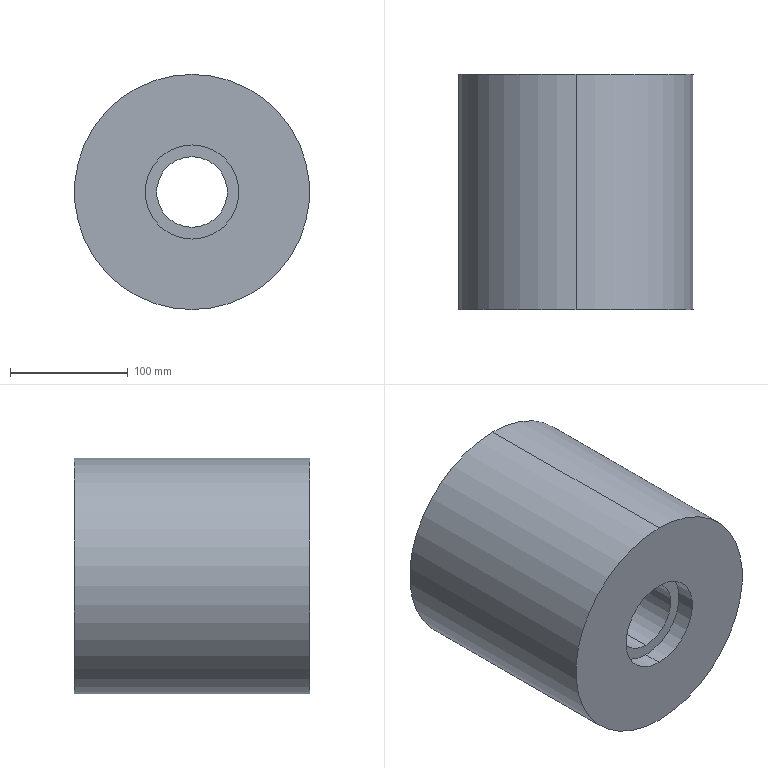Part | SolidWorks | features BaseBody 1 | 1 solid | 12 faces | box 200 x 200 x 200 mm | volume 5647327 mm3 | cylinder 8 | plane 4 | commonest cylinder face diameters 80 x4 60 x2 200 x2
STEP:
#1=CARTESIAN_POINT('',(0.,16.,40.));
#2=VERTEX_POINT('',#1);
#3=CARTESIAN_POINT('',(0.,16.,-40.));
#4=VERTEX_POINT('',#3);
#5=CARTESIAN_POINT('',(0.,16.,0.));
#6=DIRECTION('',(0.,-1.,0.));
#7=DIRECTION('',(0.,0.,-1.));
#8=AXIS2_PLACEMENT_3D('',#5,#6,#7);
#9=CIRCLE('',#8,40.);
#10=EDGE_CURVE('',#2,#4,#9,.T.);
#11=ORIENTED_EDGE('',*,*,#10,.F.);
#12=CARTESIAN_POINT('',(0.,0.,40.));
#13=VERTEX_POINT('',#12);
#14=CARTESIAN_POINT('',(0.,16.,40.));
#15=DIRECTION('',(0.,-1.,0.));
#16=VECTOR('',#15,1000.);
#17=LINE('',#14,#16);
#18=EDGE_CURVE('',#2,#13,#17,.T.);
#19=ORIENTED_EDGE('',*,*,#18,.T.);
#20=CARTESIAN_POINT('',(0.,0.,-40.));
#21=VERTEX_POINT('',#20);
#22=CARTESIAN_POINT('',(0.,0.,0.));
#23=DIRECTION('',(0.,-1.,0.));
#24=DIRECTION('',(0.,0.,-1.));
#25=AXIS2_PLACEMENT_3D('',#22,#23,#24);
#26=CIRCLE('',#25,40.);
#27=EDGE_CURVE('',#13,#21,#26,.T.);
#28=ORIENTED_EDGE('',*,*,#27,.T.);
#29=CARTESIAN_POINT('',(0.,16.,-40.));
#30=DIRECTION('',(0.,-1.,0.));
#31=VECTOR('',#30,1000.);
#32=LINE('',#29,#31);
#33=EDGE_CURVE('',#4,#21,#32,.T.);
#34=ORIENTED_EDGE('',*,*,#33,.F.);
#35=EDGE_LOOP('',(#11,#19,#28,#34));
#36=FACE_OUTER_BOUND('',#35,.T.);
#37=CARTESIAN_POINT('',(0.,16.,0.));
#38=DIRECTION('',(0.,-1.,0.));
#39=DIRECTION('',(0.,0.,-1.));
#40=AXIS2_PLACEMENT_3D('',#37,#38,#39);
#41=CYLINDRICAL_SURFACE('',#40,40.);
#42=ADVANCED_FACE('',(#36),#41,.F.);
#43=CARTESIAN_POINT('',(0.,184.,-40.));
#44=VERTEX_POINT('',#43);
#45=CARTESIAN_POINT('',(0.,184.,40.));
#46=VERTEX_POINT('',#45);
#47=CARTESIAN_POINT('',(0.,184.,0.));
#48=DIRECTION('',(0.,1.,0.));
#49=DIRECTION('',(0.,0.,1.));
#50=AXIS2_PLACEMENT_3D('',#47,#48,#49);
#51=CIRCLE('',#50,40.);
#52=EDGE_CURVE('',#44,#46,#51,.T.);
#53=ORIENTED_EDGE('',*,*,#52,.F.);
#54=CARTESIAN_POINT('',(0.,200.,-40.));
#55=VERTEX_POINT('',#54);
#56=CARTESIAN_POINT('',(0.,184.,-40.));
#57=DIRECTION('',(0.,1.,0.));
#58=VECTOR('',#57,1000.);
#59=LINE('',#56,#58);
#60=EDGE_CURVE('',#44,#55,#59,.T.);
#61=ORIENTED_EDGE('',*,*,#60,.T.);
#62=CARTESIAN_POINT('',(0.,200.,40.));
#63=VERTEX_POINT('',#62);
#64=CARTESIAN_POINT('',(0.,200.,0.));
#65=DIRECTION('',(0.,1.,0.));
#66=DIRECTION('',(0.,0.,1.));
#67=AXIS2_PLACEMENT_3D('',#64,#65,#66);
#68=CIRCLE('',#67,40.);
#69=EDGE_CURVE('',#55,#63,#68,.T.);
#70=ORIENTED_EDGE('',*,*,#69,.T.);
#71=CARTESIAN_POINT('',(0.,184.,40.));
#72=DIRECTION('',(0.,1.,0.));
#73=VECTOR('',#72,1000.);
#74=LINE('',#71,#73);
#75=EDGE_CURVE('',#46,#63,#74,.T.);
#76=ORIENTED_EDGE('',*,*,#75,.F.);
#77=EDGE_LOOP('',(#53,#61,#70,#76));
#78=FACE_OUTER_BOUND('',#77,.T.);
#79=CARTESIAN_POINT('',(0.,184.,0.));
#80=DIRECTION('',(0.,1.,0.));
#81=DIRECTION('',(0.,0.,1.));
#82=AXIS2_PLACEMENT_3D('',#79,#80,#81);
#83=CYLINDRICAL_SURFACE('',#82,40.);
#84=ADVANCED_FACE('',(#78),#83,.F.);
#85=CARTESIAN_POINT('',(0.,200.,100.));
#86=VERTEX_POINT('',#85);
#87=CARTESIAN_POINT('',(0.,200.,-100.));
#88=VERTEX_POINT('',#87);
#89=CARTESIAN_POINT('',(0.,200.,0.));
#90=DIRECTION('',(0.,1.,0.));
#91=DIRECTION('',(0.,0.,1.));
#92=AXIS2_PLACEMENT_3D('',#89,#90,#91);
#93=CIRCLE('',#92,100.);
#94=EDGE_CURVE('',#86,#88,#93,.T.);
#95=ORIENTED_EDGE('',*,*,#94,.F.);
#96=CARTESIAN_POINT('',(0.,0.,100.));
#97=VERTEX_POINT('',#96);
#98=CARTESIAN_POINT('',(0.,200.,100.));
#99=DIRECTION('',(0.,-1.,0.));
#100=VECTOR('',#99,1000.);
#101=LINE('',#98,#100);
#102=EDGE_CURVE('',#86,#97,#101,.T.);
#103=ORIENTED_EDGE('',*,*,#102,.T.);
#104=CARTESIAN_POINT('',(0.,0.,-100.));
#105=VERTEX_POINT('',#104);
#106=CARTESIAN_POINT('',(0.,0.,0.));
#107=DIRECTION('',(0.,1.,0.));
#108=DIRECTION('',(0.,0.,1.));
#109=AXIS2_PLACEMENT_3D('',#106,#107,#108);
#110=CIRCLE('',#109,100.);
#111=EDGE_CURVE('',#97,#105,#110,.T.);
#112=ORIENTED_EDGE('',*,*,#111,.T.);
#113=CARTESIAN_POINT('',(0.,200.,-100.));
#114=DIRECTION('',(0.,-1.,0.));
#115=VECTOR('',#114,1000.);
#116=LINE('',#113,#115);
#117=EDGE_CURVE('',#88,#105,#116,.T.);
#118=ORIENTED_EDGE('',*,*,#117,.F.);
#119=EDGE_LOOP('',(#95,#103,#112,#118));
#120=FACE_OUTER_BOUND('',#119,.T.);
#121=CARTESIAN_POINT('',(0.,200.,0.));
#122=DIRECTION('',(0.,-1.,0.));
#123=DIRECTION('',(0.,0.,-1.));
#124=AXIS2_PLACEMENT_3D('',#121,#122,#123);
#125=CYLINDRICAL_SURFACE('',#124,100.);
#126=ADVANCED_FACE('',(#120),#125,.T.);
#127=CARTESIAN_POINT('',(0.,16.,-30.));
#128=VERTEX_POINT('',#127);
#129=CARTESIAN_POINT('',(0.,16.,30.));
#130=VERTEX_POINT('',#129);
#131=CARTESIAN_POINT('',(0.,16.,0.));
#132=DIRECTION('',(0.,1.,0.));
#133=DIRECTION('',(0.,0.,-1.));
#134=AXIS2_PLACEMENT_3D('',#131,#132,#133);
#135=CIRCLE('',#134,30.);
#136=EDGE_CURVE('',#128,#130,#135,.T.);
#137=ORIENTED_EDGE('',*,*,#136,.F.);
#138=CARTESIAN_POINT('',(0.,184.,-30.));
#139=VERTEX_POINT('',#138);
#140=CARTESIAN_POINT('',(0.,0.,-30.));
#141=DIRECTION('',(0.,1.,0.));
#142=VECTOR('',#141,1000.);
#143=LINE('',#140,#142);
#144=EDGE_CURVE('',#128,#139,#143,.T.);
#145=ORIENTED_EDGE('',*,*,#144,.T.);
#146=CARTESIAN_POINT('',(0.,184.,30.));
#147=VERTEX_POINT('',#146);
#148=CARTESIAN_POINT('',(0.,184.,0.));
#149=DIRECTION('',(0.,-1.,0.));
#150=DIRECTION('',(0.,0.,1.));
#151=AXIS2_PLACEMENT_3D('',#148,#149,#150);
#152=CIRCLE('',#151,30.);
#153=EDGE_CURVE('',#147,#139,#152,.T.);
#154=ORIENTED_EDGE('',*,*,#153,.F.);
#155=CARTESIAN_POINT('',(0.,0.,30.));
#156=DIRECTION('',(0.,1.,0.));
#157=VECTOR('',#156,1000.);
#158=LINE('',#155,#157);
#159=EDGE_CURVE('',#130,#147,#158,.T.);
#160=ORIENTED_EDGE('',*,*,#159,.F.);
#161=EDGE_LOOP('',(#137,#145,#154,#160));
#162=FACE_OUTER_BOUND('',#161,.T.);
#163=CARTESIAN_POINT('',(0.,0.,0.));
#164=DIRECTION('',(0.,1.,0.));
#165=DIRECTION('',(0.,0.,1.));
#166=AXIS2_PLACEMENT_3D('',#163,#164,#165);
#167=CYLINDRICAL_SURFACE('',#166,30.);
#168=ADVANCED_FACE('',(#162),#167,.F.);
#169=ORIENTED_EDGE('',*,*,#144,.F.);
#170=CARTESIAN_POINT('',(0.,16.,0.));
#171=DIRECTION('',(0.,1.,0.));
#172=DIRECTION('',(0.,0.,-1.));
#173=AXIS2_PLACEMENT_3D('',#170,#171,#172);
#174=CIRCLE('',#173,30.);
#175=EDGE_CURVE('',#130,#128,#174,.T.);
#176=ORIENTED_EDGE('',*,*,#175,.F.);
#177=ORIENTED_EDGE('',*,*,#159,.T.);
#178=CARTESIAN_POINT('',(0.,184.,0.));
#179=DIRECTION('',(0.,-1.,0.));
#180=DIRECTION('',(0.,0.,1.));
#181=AXIS2_PLACEMENT_3D('',#178,#179,#180);
#182=CIRCLE('',#181,30.);
#183=EDGE_CURVE('',#139,#147,#182,.T.);
#184=ORIENTED_EDGE('',*,*,#183,.F.);
#185=EDGE_LOOP('',(#169,#176,#177,#184));
#186=FACE_OUTER_BOUND('',#185,.T.);
#187=CARTESIAN_POINT('',(0.,0.,0.));
#188=DIRECTION('',(0.,1.,0.));
#189=DIRECTION('',(0.,0.,1.));
#190=AXIS2_PLACEMENT_3D('',#187,#188,#189);
#191=CYLINDRICAL_SURFACE('',#190,30.);
#192=ADVANCED_FACE('',(#186),#191,.F.);
#193=ORIENTED_EDGE('',*,*,#102,.F.);
#194=CARTESIAN_POINT('',(0.,200.,0.));
#195=DIRECTION('',(0.,1.,0.));
#196=DIRECTION('',(0.,0.,1.));
#197=AXIS2_PLACEMENT_3D('',#194,#195,#196);
#198=CIRCLE('',#197,100.);
#199=EDGE_CURVE('',#88,#86,#198,.T.);
#200=ORIENTED_EDGE('',*,*,#199,.F.);
#201=ORIENTED_EDGE('',*,*,#117,.T.);
#202=CARTESIAN_POINT('',(0.,0.,0.));
#203=DIRECTION('',(0.,1.,0.));
#204=DIRECTION('',(0.,0.,1.));
#205=AXIS2_PLACEMENT_3D('',#202,#203,#204);
#206=CIRCLE('',#205,100.);
#207=EDGE_CURVE('',#105,#97,#206,.T.);
#208=ORIENTED_EDGE('',*,*,#207,.T.);
#209=EDGE_LOOP('',(#193,#200,#201,#208));
#210=FACE_OUTER_BOUND('',#209,.T.);
#211=CARTESIAN_POINT('',(0.,200.,0.));
#212=DIRECTION('',(0.,-1.,0.));
#213=DIRECTION('',(0.,0.,-1.));
#214=AXIS2_PLACEMENT_3D('',#211,#212,#213);
#215=CYLINDRICAL_SURFACE('',#214,100.);
#216=ADVANCED_FACE('',(#210),#215,.T.);
#217=CARTESIAN_POINT('',(0.,200.,0.));
#218=DIRECTION('',(0.,1.,0.));
#219=DIRECTION('',(0.,0.,1.));
#220=AXIS2_PLACEMENT_3D('',#217,#218,#219);
#221=CIRCLE('',#220,40.);
#222=EDGE_CURVE('',#63,#55,#221,.T.);
#223=ORIENTED_EDGE('',*,*,#222,.F.);
#224=ORIENTED_EDGE('',*,*,#69,.F.);
#225=EDGE_LOOP('',(#223,#224));
#226=FACE_BOUND('',#225,.T.);
#227=ORIENTED_EDGE('',*,*,#199,.T.);
#228=ORIENTED_EDGE('',*,*,#94,.T.);
#229=EDGE_LOOP('',(#227,#228));
#230=FACE_OUTER_BOUND('',#229,.T.);
#231=CARTESIAN_POINT('',(0.,200.,0.));
#232=DIRECTION('',(0.,1.,0.));
#233=DIRECTION('',(0.,0.,1.));
#234=AXIS2_PLACEMENT_3D('',#231,#232,#233);
#235=PLANE('',#234);
#236=ADVANCED_FACE('',(#226,#230),#235,.T.);
#237=CARTESIAN_POINT('',(0.,0.,0.));
#238=DIRECTION('',(0.,-1.,0.));
#239=DIRECTION('',(0.,0.,-1.));
#240=AXIS2_PLACEMENT_3D('',#237,#238,#239);
#241=CIRCLE('',#240,40.);
#242=EDGE_CURVE('',#21,#13,#241,.T.);
#243=ORIENTED_EDGE('',*,*,#242,.F.);
#244=ORIENTED_EDGE('',*,*,#27,.F.);
#245=EDGE_LOOP('',(#243,#244));
#246=FACE_BOUND('',#245,.T.);
#247=ORIENTED_EDGE('',*,*,#207,.F.);
#248=ORIENTED_EDGE('',*,*,#111,.F.);
#249=EDGE_LOOP('',(#247,#248));
#250=FACE_OUTER_BOUND('',#249,.T.);
#251=CARTESIAN_POINT('',(0.,0.,0.));
#252=DIRECTION('',(0.,1.,0.));
#253=DIRECTION('',(0.,0.,1.));
#254=AXIS2_PLACEMENT_3D('',#251,#252,#253);
#255=PLANE('',#254);
#256=ADVANCED_FACE('',(#246,#250),#255,.F.);
#257=CARTESIAN_POINT('',(0.,184.,0.));
#258=DIRECTION('',(0.,1.,0.));
#259=DIRECTION('',(0.,0.,1.));
#260=AXIS2_PLACEMENT_3D('',#257,#258,#259);
#261=CIRCLE('',#260,40.);
#262=EDGE_CURVE('',#46,#44,#261,.T.);
#263=ORIENTED_EDGE('',*,*,#262,.T.);
#264=ORIENTED_EDGE('',*,*,#52,.T.);
#265=EDGE_LOOP('',(#263,#264));
#266=FACE_OUTER_BOUND('',#265,.T.);
#267=ORIENTED_EDGE('',*,*,#153,.T.);
#268=ORIENTED_EDGE('',*,*,#183,.T.);
#269=EDGE_LOOP('',(#267,#268));
#270=FACE_BOUND('',#269,.T.);
#271=CARTESIAN_POINT('',(0.,184.,0.));
#272=DIRECTION('',(0.,1.,0.));
#273=DIRECTION('',(0.,0.,1.));
#274=AXIS2_PLACEMENT_3D('',#271,#272,#273);
#275=PLANE('',#274);
#276=ADVANCED_FACE('',(#266,#270),#275,.T.);
#277=ORIENTED_EDGE('',*,*,#60,.F.);
#278=ORIENTED_EDGE('',*,*,#262,.F.);
#279=ORIENTED_EDGE('',*,*,#75,.T.);
#280=ORIENTED_EDGE('',*,*,#222,.T.);
#281=EDGE_LOOP('',(#277,#278,#279,#280));
#282=FACE_OUTER_BOUND('',#281,.T.);
#283=CARTESIAN_POINT('',(0.,184.,0.));
#284=DIRECTION('',(0.,1.,0.));
#285=DIRECTION('',(0.,0.,1.));
#286=AXIS2_PLACEMENT_3D('',#283,#284,#285);
#287=CYLINDRICAL_SURFACE('',#286,40.);
#288=ADVANCED_FACE('',(#282),#287,.F.);
#289=CARTESIAN_POINT('',(0.,16.,0.));
#290=DIRECTION('',(0.,-1.,0.));
#291=DIRECTION('',(0.,0.,-1.));
#292=AXIS2_PLACEMENT_3D('',#289,#290,#291);
#293=CIRCLE('',#292,40.);
#294=EDGE_CURVE('',#4,#2,#293,.T.);
#295=ORIENTED_EDGE('',*,*,#294,.T.);
#296=ORIENTED_EDGE('',*,*,#10,.T.);
#297=EDGE_LOOP('',(#295,#296));
#298=FACE_OUTER_BOUND('',#297,.T.);
#299=ORIENTED_EDGE('',*,*,#175,.T.);
#300=ORIENTED_EDGE('',*,*,#136,.T.);
#301=EDGE_LOOP('',(#299,#300));
#302=FACE_BOUND('',#301,.T.);
#303=CARTESIAN_POINT('',(0.,16.,0.));
#304=DIRECTION('',(0.,-1.,0.));
#305=DIRECTION('',(0.,0.,-1.));
#306=AXIS2_PLACEMENT_3D('',#303,#304,#305);
#307=PLANE('',#306);
#308=ADVANCED_FACE('',(#298,#302),#307,.T.);
#309=ORIENTED_EDGE('',*,*,#18,.F.);
#310=ORIENTED_EDGE('',*,*,#294,.F.);
#311=ORIENTED_EDGE('',*,*,#33,.T.);
#312=ORIENTED_EDGE('',*,*,#242,.T.);
#313=EDGE_LOOP('',(#309,#310,#311,#312));
#314=FACE_OUTER_BOUND('',#313,.T.);
#315=CARTESIAN_POINT('',(0.,16.,0.));
#316=DIRECTION('',(0.,-1.,0.));
#317=DIRECTION('',(0.,0.,-1.));
#318=AXIS2_PLACEMENT_3D('',#315,#316,#317);
#319=CYLINDRICAL_SURFACE('',#318,40.);
#320=ADVANCED_FACE('',(#314),#319,.F.);
#321=CLOSED_SHELL('',(#42,#84,#126,#168,#192,#216,#236,#256,#276,#288,#308,#320));
#322=MANIFOLD_SOLID_BREP('',#321);
#323=CARTESIAN_POINT('',(0.,0.,0.));
#324=DIRECTION('',(0.,0.,1.));
#325=DIRECTION('',(1.,0.,0.));
#326=AXIS2_PLACEMENT_3D('',#323,#324,#325);
#327=(LENGTH_UNIT()NAMED_UNIT(*)SI_UNIT(.MILLI.,.METRE.));
#328=UNCERTAINTY_MEASURE_WITH_UNIT(LENGTH_MEASURE(0.00001),#327,'','');
#329=(NAMED_UNIT(*)PLANE_ANGLE_UNIT()SI_UNIT($,.RADIAN.));
#330=(NAMED_UNIT(*)SI_UNIT($,.STERADIAN.)SOLID_ANGLE_UNIT());
#331=(GEOMETRIC_REPRESENTATION_CONTEXT(3)GLOBAL_UNCERTAINTY_ASSIGNED_CONTEXT((#328))GLOBAL_UNIT_ASSIGNED_CONTEXT((#327,#329,#330))REPRESENTATION_CONTEXT('',''));
#332=ADVANCED_BREP_SHAPE_REPRESENTATION('',(#322,#326),#331);